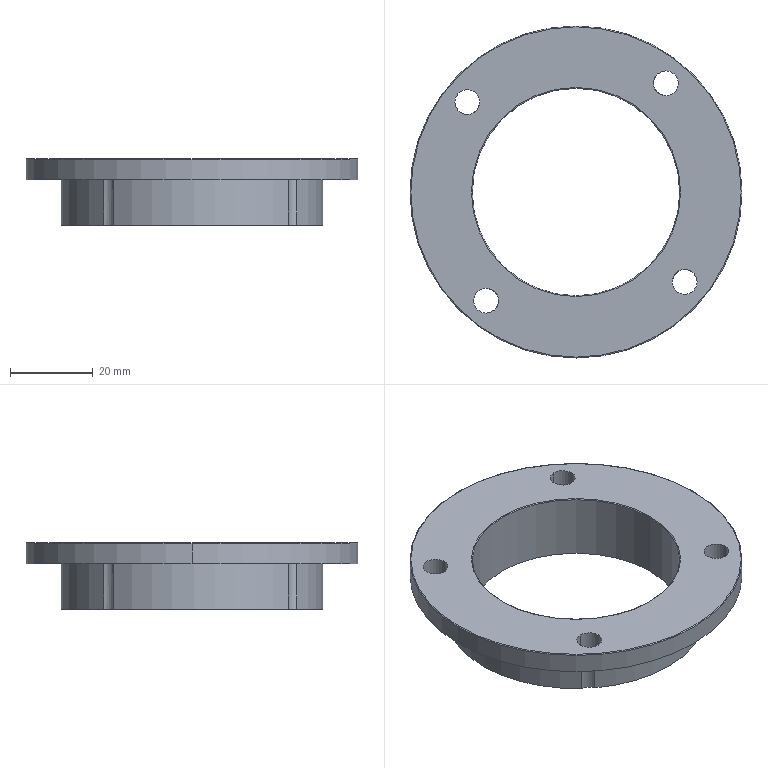Part | SolidWorks | 1 solid | 24 faces | box 80 x 80 x 16 mm | volume 27390 mm3 | cylinder 17 | torus 4 | plane 3 | commonest cylinder face diameters 6 x8 63 x5 50 x2 80 x2
STEP:
#1=CARTESIAN_POINT('',(325.,0.,69.8));
#2=VERTEX_POINT('',#1);
#3=CARTESIAN_POINT('',(275.,0.,69.8));
#4=VERTEX_POINT('',#3);
#5=CARTESIAN_POINT('',(300.,0.,69.8));
#6=DIRECTION('',(0.,0.,1.));
#7=DIRECTION('',(1.,0.009983,0.));
#8=AXIS2_PLACEMENT_3D('',#5,#6,#7);
#9=CIRCLE('',#8,25.);
#10=EDGE_CURVE('',#2,#4,#9,.T.);
#11=ORIENTED_EDGE('',*,*,#10,.F.);
#12=CARTESIAN_POINT('',(325.2,0.,70.));
#13=VERTEX_POINT('',#12);
#14=CARTESIAN_POINT('',(325.2,0.,69.8));
#15=DIRECTION('',(0.,1.,0.));
#16=DIRECTION('',(-1.,0.,0.));
#17=AXIS2_PLACEMENT_3D('',#14,#15,#16);
#18=CIRCLE('',#17,0.2);
#19=EDGE_CURVE('',#2,#13,#18,.T.);
#20=ORIENTED_EDGE('',*,*,#19,.T.);
#21=CARTESIAN_POINT('',(274.8,0.,70.));
#22=VERTEX_POINT('',#21);
#23=CARTESIAN_POINT('',(300.,0.,70.));
#24=DIRECTION('',(0.,0.,1.));
#25=DIRECTION('',(1.,0.,0.));
#26=AXIS2_PLACEMENT_3D('',#23,#24,#25);
#27=CIRCLE('',#26,25.2);
#28=EDGE_CURVE('',#13,#22,#27,.T.);
#29=ORIENTED_EDGE('',*,*,#28,.T.);
#30=CARTESIAN_POINT('',(274.8,0.,69.8));
#31=DIRECTION('',(0.,-1.,0.));
#32=DIRECTION('',(1.,0.,0.));
#33=AXIS2_PLACEMENT_3D('',#30,#31,#32);
#34=CIRCLE('',#33,0.2);
#35=EDGE_CURVE('',#4,#22,#34,.T.);
#36=ORIENTED_EDGE('',*,*,#35,.F.);
#37=EDGE_LOOP('',(#11,#20,#29,#36));
#38=FACE_OUTER_BOUND('',#37,.T.);
#39=CARTESIAN_POINT('',(300.,0.,69.8));
#40=DIRECTION('',(0.,0.,1.));
#41=DIRECTION('',(-1.,-0.009983,0.));
#42=AXIS2_PLACEMENT_3D('',#39,#40,#41);
#43=TOROIDAL_SURFACE('',#42,25.2,0.2);
#44=ADVANCED_FACE('',(#38),#43,.T.);
#45=CARTESIAN_POINT('',(300.,0.,69.8));
#46=DIRECTION('',(0.,0.,1.));
#47=DIRECTION('',(-1.,-0.009983,0.));
#48=AXIS2_PLACEMENT_3D('',#45,#46,#47);
#49=CIRCLE('',#48,25.);
#50=EDGE_CURVE('',#4,#2,#49,.T.);
#51=ORIENTED_EDGE('',*,*,#50,.F.);
#52=ORIENTED_EDGE('',*,*,#35,.T.);
#53=CARTESIAN_POINT('',(300.,0.,70.));
#54=DIRECTION('',(0.,0.,1.));
#55=DIRECTION('',(-1.,0.,0.));
#56=AXIS2_PLACEMENT_3D('',#53,#54,#55);
#57=CIRCLE('',#56,25.2);
#58=EDGE_CURVE('',#22,#13,#57,.T.);
#59=ORIENTED_EDGE('',*,*,#58,.T.);
#60=ORIENTED_EDGE('',*,*,#19,.F.);
#61=EDGE_LOOP('',(#51,#52,#59,#60));
#62=FACE_OUTER_BOUND('',#61,.T.);
#63=CARTESIAN_POINT('',(300.,0.,69.8));
#64=DIRECTION('',(0.,0.,1.));
#65=DIRECTION('',(1.,0.009983,0.));
#66=AXIS2_PLACEMENT_3D('',#63,#64,#65);
#67=TOROIDAL_SURFACE('',#66,25.2,0.2);
#68=ADVANCED_FACE('',(#62),#67,.T.);
#69=CARTESIAN_POINT('',(325.,0.,54.));
#70=VERTEX_POINT('',#69);
#71=CARTESIAN_POINT('',(275.,0.,54.));
#72=VERTEX_POINT('',#71);
#73=CARTESIAN_POINT('',(300.,0.,54.));
#74=DIRECTION('',(0.,0.,-1.));
#75=DIRECTION('',(1.,0.,0.));
#76=AXIS2_PLACEMENT_3D('',#73,#74,#75);
#77=CIRCLE('',#76,25.);
#78=EDGE_CURVE('',#70,#72,#77,.T.);
#79=ORIENTED_EDGE('',*,*,#78,.T.);
#80=CARTESIAN_POINT('',(275.,0.,54.));
#81=DIRECTION('',(0.,0.,1.));
#82=VECTOR('',#81,1000.);
#83=LINE('',#80,#82);
#84=EDGE_CURVE('',#72,#4,#83,.T.);
#85=ORIENTED_EDGE('',*,*,#84,.T.);
#86=ORIENTED_EDGE('',*,*,#50,.T.);
#87=CARTESIAN_POINT('',(325.,0.,54.));
#88=DIRECTION('',(0.,0.,1.));
#89=VECTOR('',#88,1000.);
#90=LINE('',#87,#89);
#91=EDGE_CURVE('',#70,#2,#90,.T.);
#92=ORIENTED_EDGE('',*,*,#91,.F.);
#93=EDGE_LOOP('',(#79,#85,#86,#92));
#94=FACE_OUTER_BOUND('',#93,.T.);
#95=CARTESIAN_POINT('',(300.,0.,70.));
#96=DIRECTION('',(0.,0.,1.));
#97=DIRECTION('',(1.,0.,0.));
#98=AXIS2_PLACEMENT_3D('',#95,#96,#97);
#99=CYLINDRICAL_SURFACE('',#98,25.);
#100=ADVANCED_FACE('',(#94),#99,.F.);
#101=CARTESIAN_POINT('',(300.,0.,54.));
#102=DIRECTION('',(0.,0.,-1.));
#103=DIRECTION('',(-1.,0.,0.));
#104=AXIS2_PLACEMENT_3D('',#101,#102,#103);
#105=CIRCLE('',#104,25.);
#106=EDGE_CURVE('',#72,#70,#105,.T.);
#107=ORIENTED_EDGE('',*,*,#106,.T.);
#108=ORIENTED_EDGE('',*,*,#91,.T.);
#109=ORIENTED_EDGE('',*,*,#10,.T.);
#110=ORIENTED_EDGE('',*,*,#84,.F.);
#111=EDGE_LOOP('',(#107,#108,#109,#110));
#112=FACE_OUTER_BOUND('',#111,.T.);
#113=CARTESIAN_POINT('',(300.,0.,70.));
#114=DIRECTION('',(0.,0.,1.));
#115=DIRECTION('',(1.,0.,0.));
#116=AXIS2_PLACEMENT_3D('',#113,#114,#115);
#117=CYLINDRICAL_SURFACE('',#116,25.);
#118=ADVANCED_FACE('',(#112),#117,.F.);
#119=CARTESIAN_POINT('',(331.5,0.,54.));
#120=VERTEX_POINT('',#119);
#121=CARTESIAN_POINT('',(321.283,23.223,54.));
#122=VERTEX_POINT('',#121);
#123=CARTESIAN_POINT('',(300.,0.,54.));
#124=DIRECTION('',(0.,0.,1.));
#125=DIRECTION('',(1.,0.,0.));
#126=AXIS2_PLACEMENT_3D('',#123,#124,#125);
#127=CIRCLE('',#126,31.5);
#128=EDGE_CURVE('',#120,#122,#127,.T.);
#129=ORIENTED_EDGE('',*,*,#128,.T.);
#130=CARTESIAN_POINT('',(321.283,23.223,65.));
#131=VERTEX_POINT('',#130);
#132=CARTESIAN_POINT('',(321.283,23.223,54.));
#133=DIRECTION('',(0.,0.,1.));
#134=VECTOR('',#133,1000.);
#135=LINE('',#132,#134);
#136=EDGE_CURVE('',#122,#131,#135,.T.);
#137=ORIENTED_EDGE('',*,*,#136,.T.);
#138=CARTESIAN_POINT('',(331.5,0.,65.));
#139=VERTEX_POINT('',#138);
#140=CARTESIAN_POINT('',(300.,0.,65.));
#141=DIRECTION('',(0.,0.,-1.));
#142=DIRECTION('',(0.6756,0.7372,0.));
#143=AXIS2_PLACEMENT_3D('',#140,#141,#142);
#144=CIRCLE('',#143,31.5);
#145=EDGE_CURVE('',#131,#139,#144,.T.);
#146=ORIENTED_EDGE('',*,*,#145,.T.);
#147=CARTESIAN_POINT('',(331.5,0.,65.));
#148=DIRECTION('',(0.,0.,-1.));
#149=VECTOR('',#148,1000.);
#150=LINE('',#147,#149);
#151=EDGE_CURVE('',#139,#120,#150,.T.);
#152=ORIENTED_EDGE('',*,*,#151,.T.);
#153=EDGE_LOOP('',(#129,#137,#146,#152));
#154=FACE_OUTER_BOUND('',#153,.T.);
#155=CARTESIAN_POINT('',(300.,0.,70.));
#156=DIRECTION('',(0.,0.,1.));
#157=DIRECTION('',(1.,0.,0.));
#158=AXIS2_PLACEMENT_3D('',#155,#156,#157);
#159=CYLINDRICAL_SURFACE('',#158,31.5);
#160=ADVANCED_FACE('',(#154),#159,.T.);
#161=ORIENTED_EDGE('',*,*,#151,.F.);
#162=CARTESIAN_POINT('',(325.257,-18.824,65.));
#163=VERTEX_POINT('',#162);
#164=CARTESIAN_POINT('',(300.,0.,65.));
#165=DIRECTION('',(0.,0.,-1.));
#166=DIRECTION('',(1.,0.,0.));
#167=AXIS2_PLACEMENT_3D('',#164,#165,#166);
#168=CIRCLE('',#167,31.5);
#169=EDGE_CURVE('',#139,#163,#168,.T.);
#170=ORIENTED_EDGE('',*,*,#169,.T.);
#171=CARTESIAN_POINT('',(325.257,-18.824,54.));
#172=VERTEX_POINT('',#171);
#173=CARTESIAN_POINT('',(325.257,-18.824,65.));
#174=DIRECTION('',(0.,0.,-1.));
#175=VECTOR('',#174,1000.);
#176=LINE('',#173,#175);
#177=EDGE_CURVE('',#163,#172,#176,.T.);
#178=ORIENTED_EDGE('',*,*,#177,.T.);
#179=CARTESIAN_POINT('',(300.,0.,54.));
#180=DIRECTION('',(0.,0.,1.));
#181=DIRECTION('',(0.8018,-0.5976,0.));
#182=AXIS2_PLACEMENT_3D('',#179,#180,#181);
#183=CIRCLE('',#182,31.5);
#184=EDGE_CURVE('',#172,#120,#183,.T.);
#185=ORIENTED_EDGE('',*,*,#184,.T.);
#186=EDGE_LOOP('',(#161,#170,#178,#185));
#187=FACE_OUTER_BOUND('',#186,.T.);
#188=CARTESIAN_POINT('',(300.,0.,70.));
#189=DIRECTION('',(0.,0.,1.));
#190=DIRECTION('',(1.,0.,0.));
#191=AXIS2_PLACEMENT_3D('',#188,#189,#190);
#192=CYLINDRICAL_SURFACE('',#191,31.5);
#193=ADVANCED_FACE('',(#187),#192,.T.);
#194=CARTESIAN_POINT('',(323.197,-21.672,70.));
#195=VERTEX_POINT('',#194);
#196=CARTESIAN_POINT('',(329.197,-21.672,70.));
#197=VERTEX_POINT('',#196);
#198=CARTESIAN_POINT('',(326.197,-21.672,70.));
#199=DIRECTION('',(0.,0.,1.));
#200=DIRECTION('',(-1.,0.,0.));
#201=AXIS2_PLACEMENT_3D('',#198,#199,#200);
#202=CIRCLE('',#201,3.);
#203=EDGE_CURVE('',#195,#197,#202,.T.);
#204=ORIENTED_EDGE('',*,*,#203,.T.);
#205=CARTESIAN_POINT('',(329.197,-21.672,65.));
#206=VERTEX_POINT('',#205);
#207=CARTESIAN_POINT('',(329.197,-21.672,65.));
#208=DIRECTION('',(0.,0.,1.));
#209=VECTOR('',#208,1000.);
#210=LINE('',#207,#209);
#211=EDGE_CURVE('',#206,#197,#210,.T.);
#212=ORIENTED_EDGE('',*,*,#211,.F.);
#213=CARTESIAN_POINT('',(323.197,-21.672,65.));
#214=VERTEX_POINT('',#213);
#215=CARTESIAN_POINT('',(326.197,-21.672,65.));
#216=DIRECTION('',(0.,0.,-1.));
#217=DIRECTION('',(1.,0.,0.));
#218=AXIS2_PLACEMENT_3D('',#215,#216,#217);
#219=CIRCLE('',#218,3.);
#220=EDGE_CURVE('',#206,#214,#219,.T.);
#221=ORIENTED_EDGE('',*,*,#220,.T.);
#222=CARTESIAN_POINT('',(323.197,-21.672,65.));
#223=DIRECTION('',(0.,0.,1.));
#224=VECTOR('',#223,1000.);
#225=LINE('',#222,#224);
#226=EDGE_CURVE('',#214,#195,#225,.T.);
#227=ORIENTED_EDGE('',*,*,#226,.T.);
#228=EDGE_LOOP('',(#204,#212,#221,#227));
#229=FACE_OUTER_BOUND('',#228,.T.);
#230=CARTESIAN_POINT('',(326.197,-21.672,70.));
#231=DIRECTION('',(0.,0.,1.));
#232=DIRECTION('',(-1.,0.,0.));
#233=AXIS2_PLACEMENT_3D('',#230,#231,#232);
#234=CYLINDRICAL_SURFACE('',#233,3.);
#235=ADVANCED_FACE('',(#229),#234,.F.);
#236=CARTESIAN_POINT('',(326.197,-21.672,70.));
#237=DIRECTION('',(0.,0.,1.));
#238=DIRECTION('',(1.,0.,0.));
#239=AXIS2_PLACEMENT_3D('',#236,#237,#238);
#240=CIRCLE('',#239,3.);
#241=EDGE_CURVE('',#197,#195,#240,.T.);
#242=ORIENTED_EDGE('',*,*,#241,.T.);
#243=ORIENTED_EDGE('',*,*,#226,.F.);
#244=CARTESIAN_POINT('',(323.223,-21.283,65.));
#245=VERTEX_POINT('',#244);
#246=CARTESIAN_POINT('',(326.197,-21.672,65.));
#247=DIRECTION('',(0.,0.,-1.));
#248=DIRECTION('',(-1.,0.,0.));
#249=AXIS2_PLACEMENT_3D('',#246,#247,#248);
#250=CIRCLE('',#249,3.);
#251=EDGE_CURVE('',#214,#245,#250,.T.);
#252=ORIENTED_EDGE('',*,*,#251,.T.);
#253=CARTESIAN_POINT('',(323.223,-21.283,54.));
#254=VERTEX_POINT('',#253);
#255=CARTESIAN_POINT('',(323.223,-21.283,54.));
#256=DIRECTION('',(0.,0.,1.));
#257=VECTOR('',#256,1000.);
#258=LINE('',#255,#257);
#259=EDGE_CURVE('',#254,#245,#258,.T.);
#260=ORIENTED_EDGE('',*,*,#259,.F.);
#261=CARTESIAN_POINT('',(326.197,-21.672,54.));
#262=DIRECTION('',(0.,0.,-1.));
#263=DIRECTION('',(-0.9915,0.13,0.));
#264=AXIS2_PLACEMENT_3D('',#261,#262,#263);
#265=CIRCLE('',#264,3.);
#266=EDGE_CURVE('',#254,#172,#265,.T.);
#267=ORIENTED_EDGE('',*,*,#266,.T.);
#268=ORIENTED_EDGE('',*,*,#177,.F.);
#269=CARTESIAN_POINT('',(326.197,-21.672,65.));
#270=DIRECTION('',(0.,0.,-1.));
#271=DIRECTION('',(-0.3134,0.9496,0.));
#272=AXIS2_PLACEMENT_3D('',#269,#270,#271);
#273=CIRCLE('',#272,3.);
#274=EDGE_CURVE('',#163,#206,#273,.T.);
#275=ORIENTED_EDGE('',*,*,#274,.T.);
#276=ORIENTED_EDGE('',*,*,#211,.T.);
#277=EDGE_LOOP('',(#242,#243,#252,#260,#267,#268,#275,#276));
#278=FACE_OUTER_BOUND('',#277,.T.);
#279=CARTESIAN_POINT('',(326.197,-21.672,70.));
#280=DIRECTION('',(0.,0.,1.));
#281=DIRECTION('',(-1.,0.,0.));
#282=AXIS2_PLACEMENT_3D('',#279,#280,#281);
#283=CYLINDRICAL_SURFACE('',#282,3.);
#284=ADVANCED_FACE('',(#278),#283,.F.);
#285=ORIENTED_EDGE('',*,*,#78,.F.);
#286=ORIENTED_EDGE('',*,*,#106,.F.);
#287=EDGE_LOOP('',(#285,#286));
#288=FACE_BOUND('',#287,.T.);
#289=CARTESIAN_POINT('',(274.743,18.824,54.));
#290=VERTEX_POINT('',#289);
#291=CARTESIAN_POINT('',(278.717,-23.223,54.));
#292=VERTEX_POINT('',#291);
#293=CARTESIAN_POINT('',(300.,0.,54.));
#294=DIRECTION('',(0.,0.,1.));
#295=DIRECTION('',(-1.,0.,0.));
#296=AXIS2_PLACEMENT_3D('',#293,#294,#295);
#297=CIRCLE('',#296,31.5);
#298=EDGE_CURVE('',#290,#292,#297,.T.);
#299=ORIENTED_EDGE('',*,*,#298,.F.);
#300=CARTESIAN_POINT('',(276.777,21.283,54.));
#301=VERTEX_POINT('',#300);
#302=CARTESIAN_POINT('',(273.803,21.672,54.));
#303=DIRECTION('',(0.,0.,-1.));
#304=DIRECTION('',(0.9915,-0.13,0.));
#305=AXIS2_PLACEMENT_3D('',#302,#303,#304);
#306=CIRCLE('',#305,3.);
#307=EDGE_CURVE('',#301,#290,#306,.T.);
#308=ORIENTED_EDGE('',*,*,#307,.F.);
#309=CARTESIAN_POINT('',(318.824,25.257,54.));
#310=VERTEX_POINT('',#309);
#311=CARTESIAN_POINT('',(300.,0.,54.));
#312=DIRECTION('',(0.,0.,1.));
#313=DIRECTION('',(0.5976,0.8018,0.));
#314=AXIS2_PLACEMENT_3D('',#311,#312,#313);
#315=CIRCLE('',#314,31.5);
#316=EDGE_CURVE('',#310,#301,#315,.T.);
#317=ORIENTED_EDGE('',*,*,#316,.F.);
#318=CARTESIAN_POINT('',(321.672,26.197,54.));
#319=DIRECTION('',(0.,0.,-1.));
#320=DIRECTION('',(-0.13,-0.9915,0.));
#321=AXIS2_PLACEMENT_3D('',#318,#319,#320);
#322=CIRCLE('',#321,3.);
#323=EDGE_CURVE('',#122,#310,#322,.T.);
#324=ORIENTED_EDGE('',*,*,#323,.F.);
#325=ORIENTED_EDGE('',*,*,#128,.F.);
#326=ORIENTED_EDGE('',*,*,#184,.F.);
#327=ORIENTED_EDGE('',*,*,#266,.F.);
#328=CARTESIAN_POINT('',(281.176,-25.257,54.));
#329=VERTEX_POINT('',#328);
#330=CARTESIAN_POINT('',(300.,0.,54.));
#331=DIRECTION('',(0.,0.,1.));
#332=DIRECTION('',(-0.5976,-0.8018,0.));
#333=AXIS2_PLACEMENT_3D('',#330,#331,#332);
#334=CIRCLE('',#333,31.5);
#335=EDGE_CURVE('',#329,#254,#334,.T.);
#336=ORIENTED_EDGE('',*,*,#335,.F.);
#337=CARTESIAN_POINT('',(278.328,-26.197,54.));
#338=DIRECTION('',(0.,0.,-1.));
#339=DIRECTION('',(0.13,0.9915,0.));
#340=AXIS2_PLACEMENT_3D('',#337,#338,#339);
#341=CIRCLE('',#340,3.);
#342=EDGE_CURVE('',#292,#329,#341,.T.);
#343=ORIENTED_EDGE('',*,*,#342,.F.);
#344=EDGE_LOOP('',(#299,#308,#317,#324,#325,#326,#327,#336,#343));
#345=FACE_OUTER_BOUND('',#344,.T.);
#346=CARTESIAN_POINT('',(300.497,29.496,54.));
#347=DIRECTION('',(0.,0.,1.));
#348=DIRECTION('',(1.,0.,0.));
#349=AXIS2_PLACEMENT_3D('',#346,#347,#348);
#350=PLANE('',#349);
#351=ADVANCED_FACE('',(#288,#345),#350,.F.);
#352=CARTESIAN_POINT('',(278.717,-23.223,65.));
#353=VERTEX_POINT('',#352);
#354=CARTESIAN_POINT('',(274.743,18.824,65.));
#355=VERTEX_POINT('',#354);
#356=CARTESIAN_POINT('',(300.,0.,65.));
#357=DIRECTION('',(0.,0.,-1.));
#358=DIRECTION('',(-0.6756,-0.7372,0.));
#359=AXIS2_PLACEMENT_3D('',#356,#357,#358);
#360=CIRCLE('',#359,31.5);
#361=EDGE_CURVE('',#353,#355,#360,.T.);
#362=ORIENTED_EDGE('',*,*,#361,.T.);
#363=CARTESIAN_POINT('',(274.743,18.824,65.));
#364=DIRECTION('',(0.,0.,-1.));
#365=VECTOR('',#364,1000.);
#366=LINE('',#363,#365);
#367=EDGE_CURVE('',#355,#290,#366,.T.);
#368=ORIENTED_EDGE('',*,*,#367,.T.);
#369=ORIENTED_EDGE('',*,*,#298,.T.);
#370=CARTESIAN_POINT('',(278.717,-23.223,54.));
#371=DIRECTION('',(0.,0.,1.));
#372=VECTOR('',#371,1000.);
#373=LINE('',#370,#372);
#374=EDGE_CURVE('',#292,#353,#373,.T.);
#375=ORIENTED_EDGE('',*,*,#374,.T.);
#376=EDGE_LOOP('',(#362,#368,#369,#375));
#377=FACE_OUTER_BOUND('',#376,.T.);
#378=CARTESIAN_POINT('',(300.,0.,70.));
#379=DIRECTION('',(0.,0.,1.));
#380=DIRECTION('',(1.,0.,0.));
#381=AXIS2_PLACEMENT_3D('',#378,#379,#380);
#382=CYLINDRICAL_SURFACE('',#381,31.5);
#383=ADVANCED_FACE('',(#377),#382,.T.);
#384=CARTESIAN_POINT('',(276.803,21.672,70.));
#385=VERTEX_POINT('',#384);
#386=CARTESIAN_POINT('',(270.803,21.672,70.));
#387=VERTEX_POINT('',#386);
#388=CARTESIAN_POINT('',(273.803,21.672,70.));
#389=DIRECTION('',(0.,0.,1.));
#390=DIRECTION('',(1.,0.,0.));
#391=AXIS2_PLACEMENT_3D('',#388,#389,#390);
#392=CIRCLE('',#391,3.);
#393=EDGE_CURVE('',#385,#387,#392,.T.);
#394=ORIENTED_EDGE('',*,*,#393,.T.);
#395=CARTESIAN_POINT('',(270.803,21.672,65.));
#396=VERTEX_POINT('',#395);
#397=CARTESIAN_POINT('',(270.803,21.672,65.));
#398=DIRECTION('',(0.,0.,1.));
#399=VECTOR('',#398,1000.);
#400=LINE('',#397,#399);
#401=EDGE_CURVE('',#396,#387,#400,.T.);
#402=ORIENTED_EDGE('',*,*,#401,.F.);
#403=CARTESIAN_POINT('',(276.803,21.672,65.));
#404=VERTEX_POINT('',#403);
#405=CARTESIAN_POINT('',(273.803,21.672,65.));
#406=DIRECTION('',(0.,0.,-1.));
#407=DIRECTION('',(-1.,0.,0.));
#408=AXIS2_PLACEMENT_3D('',#405,#406,#407);
#409=CIRCLE('',#408,3.);
#410=EDGE_CURVE('',#396,#404,#409,.T.);
#411=ORIENTED_EDGE('',*,*,#410,.T.);
#412=CARTESIAN_POINT('',(276.803,21.672,65.));
#413=DIRECTION('',(0.,0.,1.));
#414=VECTOR('',#413,1000.);
#415=LINE('',#412,#414);
#416=EDGE_CURVE('',#404,#385,#415,.T.);
#417=ORIENTED_EDGE('',*,*,#416,.T.);
#418=EDGE_LOOP('',(#394,#402,#411,#417));
#419=FACE_OUTER_BOUND('',#418,.T.);
#420=CARTESIAN_POINT('',(273.803,21.672,70.));
#421=DIRECTION('',(0.,0.,1.));
#422=DIRECTION('',(1.,0.,0.));
#423=AXIS2_PLACEMENT_3D('',#420,#421,#422);
#424=CYLINDRICAL_SURFACE('',#423,3.);
#425=ADVANCED_FACE('',(#419),#424,.F.);
#426=CARTESIAN_POINT('',(273.803,21.672,70.));
#427=DIRECTION('',(0.,0.,1.));
#428=DIRECTION('',(-1.,0.,0.));
#429=AXIS2_PLACEMENT_3D('',#426,#427,#428);
#430=CIRCLE('',#429,3.);
#431=EDGE_CURVE('',#387,#385,#430,.T.);
#432=ORIENTED_EDGE('',*,*,#431,.T.);
#433=ORIENTED_EDGE('',*,*,#416,.F.);
#434=CARTESIAN_POINT('',(276.777,21.283,65.));
#435=VERTEX_POINT('',#434);
#436=CARTESIAN_POINT('',(273.803,21.672,65.));
#437=DIRECTION('',(0.,0.,-1.));
#438=DIRECTION('',(1.,0.,0.));
#439=AXIS2_PLACEMENT_3D('',#436,#437,#438);
#440=CIRCLE('',#439,3.);
#441=EDGE_CURVE('',#404,#435,#440,.T.);
#442=ORIENTED_EDGE('',*,*,#441,.T.);
#443=CARTESIAN_POINT('',(276.777,21.283,54.));
#444=DIRECTION('',(0.,0.,1.));
#445=VECTOR('',#444,1000.);
#446=LINE('',#443,#445);
#447=EDGE_CURVE('',#301,#435,#446,.T.);
#448=ORIENTED_EDGE('',*,*,#447,.F.);
#449=ORIENTED_EDGE('',*,*,#307,.T.);
#450=ORIENTED_EDGE('',*,*,#367,.F.);
#451=CARTESIAN_POINT('',(273.803,21.672,65.));
#452=DIRECTION('',(0.,0.,-1.));
#453=DIRECTION('',(0.3134,-0.9496,0.));
#454=AXIS2_PLACEMENT_3D('',#451,#452,#453);
#455=CIRCLE('',#454,3.);
#456=EDGE_CURVE('',#355,#396,#455,.T.);
#457=ORIENTED_EDGE('',*,*,#456,.T.);
#458=ORIENTED_EDGE('',*,*,#401,.T.);
#459=EDGE_LOOP('',(#432,#433,#442,#448,#449,#450,#457,#458));
#460=FACE_OUTER_BOUND('',#459,.T.);
#461=CARTESIAN_POINT('',(273.803,21.672,70.));
#462=DIRECTION('',(0.,0.,1.));
#463=DIRECTION('',(1.,0.,0.));
#464=AXIS2_PLACEMENT_3D('',#461,#462,#463);
#465=CYLINDRICAL_SURFACE('',#464,3.);
#466=ADVANCED_FACE('',(#460),#465,.F.);
#467=ORIENTED_EDGE('',*,*,#316,.T.);
#468=ORIENTED_EDGE('',*,*,#447,.T.);
#469=CARTESIAN_POINT('',(318.824,25.257,65.));
#470=VERTEX_POINT('',#469);
#471=CARTESIAN_POINT('',(300.,0.,65.));
#472=DIRECTION('',(0.,0.,-1.));
#473=DIRECTION('',(-0.7372,0.6756,0.));
#474=AXIS2_PLACEMENT_3D('',#471,#472,#473);
#475=CIRCLE('',#474,31.5);
#476=EDGE_CURVE('',#435,#470,#475,.T.);
#477=ORIENTED_EDGE('',*,*,#476,.T.);
#478=CARTESIAN_POINT('',(318.824,25.257,65.));
#479=DIRECTION('',(0.,0.,-1.));
#480=VECTOR('',#479,1000.);
#481=LINE('',#478,#480);
#482=EDGE_CURVE('',#470,#310,#481,.T.);
#483=ORIENTED_EDGE('',*,*,#482,.T.);
#484=EDGE_LOOP('',(#467,#468,#477,#483));
#485=FACE_OUTER_BOUND('',#484,.T.);
#486=CARTESIAN_POINT('',(300.,0.,70.));
#487=DIRECTION('',(0.,0.,1.));
#488=DIRECTION('',(1.,0.,0.));
#489=AXIS2_PLACEMENT_3D('',#486,#487,#488);
#490=CYLINDRICAL_SURFACE('',#489,31.5);
#491=ADVANCED_FACE('',(#485),#490,.T.);
#492=CARTESIAN_POINT('',(321.672,23.197,70.));
#493=VERTEX_POINT('',#492);
#494=CARTESIAN_POINT('',(321.672,29.197,70.));
#495=VERTEX_POINT('',#494);
#496=CARTESIAN_POINT('',(321.672,26.197,70.));
#497=DIRECTION('',(0.,0.,1.));
#498=DIRECTION('',(0.,-1.,0.));
#499=AXIS2_PLACEMENT_3D('',#496,#497,#498);
#500=CIRCLE('',#499,3.);
#501=EDGE_CURVE('',#493,#495,#500,.T.);
#502=ORIENTED_EDGE('',*,*,#501,.T.);
#503=CARTESIAN_POINT('',(321.672,29.197,65.));
#504=VERTEX_POINT('',#503);
#505=CARTESIAN_POINT('',(321.672,29.197,65.));
#506=DIRECTION('',(0.,0.,1.));
#507=VECTOR('',#506,1000.);
#508=LINE('',#505,#507);
#509=EDGE_CURVE('',#504,#495,#508,.T.);
#510=ORIENTED_EDGE('',*,*,#509,.F.);
#511=CARTESIAN_POINT('',(321.672,23.197,65.));
#512=VERTEX_POINT('',#511);
#513=CARTESIAN_POINT('',(321.672,26.197,65.));
#514=DIRECTION('',(0.,0.,-1.));
#515=DIRECTION('',(0.,1.,0.));
#516=AXIS2_PLACEMENT_3D('',#513,#514,#515);
#517=CIRCLE('',#516,3.);
#518=EDGE_CURVE('',#504,#512,#517,.T.);
#519=ORIENTED_EDGE('',*,*,#518,.T.);
#520=CARTESIAN_POINT('',(321.672,23.197,65.));
#521=DIRECTION('',(0.,0.,1.));
#522=VECTOR('',#521,1000.);
#523=LINE('',#520,#522);
#524=EDGE_CURVE('',#512,#493,#523,.T.);
#525=ORIENTED_EDGE('',*,*,#524,.T.);
#526=EDGE_LOOP('',(#502,#510,#519,#525));
#527=FACE_OUTER_BOUND('',#526,.T.);
#528=CARTESIAN_POINT('',(321.672,26.197,70.));
#529=DIRECTION('',(0.,0.,1.));
#530=DIRECTION('',(0.,-1.,0.));
#531=AXIS2_PLACEMENT_3D('',#528,#529,#530);
#532=CYLINDRICAL_SURFACE('',#531,3.);
#533=ADVANCED_FACE('',(#527),#532,.F.);
#534=CARTESIAN_POINT('',(321.672,26.197,70.));
#535=DIRECTION('',(0.,0.,1.));
#536=DIRECTION('',(0.,1.,0.));
#537=AXIS2_PLACEMENT_3D('',#534,#535,#536);
#538=CIRCLE('',#537,3.);
#539=EDGE_CURVE('',#495,#493,#538,.T.);
#540=ORIENTED_EDGE('',*,*,#539,.T.);
#541=ORIENTED_EDGE('',*,*,#524,.F.);
#542=CARTESIAN_POINT('',(321.672,26.197,65.));
#543=DIRECTION('',(0.,0.,-1.));
#544=DIRECTION('',(0.,-1.,0.));
#545=AXIS2_PLACEMENT_3D('',#542,#543,#544);
#546=CIRCLE('',#545,3.);
#547=EDGE_CURVE('',#512,#131,#546,.T.);
#548=ORIENTED_EDGE('',*,*,#547,.T.);
#549=ORIENTED_EDGE('',*,*,#136,.F.);
#550=ORIENTED_EDGE('',*,*,#323,.T.);
#551=ORIENTED_EDGE('',*,*,#482,.F.);
#552=CARTESIAN_POINT('',(321.672,26.197,65.));
#553=DIRECTION('',(0.,0.,-1.));
#554=DIRECTION('',(-0.9496,-0.3134,0.));
#555=AXIS2_PLACEMENT_3D('',#552,#553,#554);
#556=CIRCLE('',#555,3.);
#557=EDGE_CURVE('',#470,#504,#556,.T.);
#558=ORIENTED_EDGE('',*,*,#557,.T.);
#559=ORIENTED_EDGE('',*,*,#509,.T.);
#560=EDGE_LOOP('',(#540,#541,#548,#549,#550,#551,#558,#559));
#561=FACE_OUTER_BOUND('',#560,.T.);
#562=CARTESIAN_POINT('',(321.672,26.197,70.));
#563=DIRECTION('',(0.,0.,1.));
#564=DIRECTION('',(0.,-1.,0.));
#565=AXIS2_PLACEMENT_3D('',#562,#563,#564);
#566=CYLINDRICAL_SURFACE('',#565,3.);
#567=ADVANCED_FACE('',(#561),#566,.F.);
#568=ORIENTED_EDGE('',*,*,#58,.F.);
#569=ORIENTED_EDGE('',*,*,#28,.F.);
#570=EDGE_LOOP('',(#568,#569));
#571=FACE_BOUND('',#570,.T.);
#572=ORIENTED_EDGE('',*,*,#393,.F.);
#573=ORIENTED_EDGE('',*,*,#431,.F.);
#574=EDGE_LOOP('',(#572,#573));
#575=FACE_BOUND('',#574,.T.);
#576=CARTESIAN_POINT('',(278.328,-23.197,70.));
#577=VERTEX_POINT('',#576);
#578=CARTESIAN_POINT('',(278.328,-29.197,70.));
#579=VERTEX_POINT('',#578);
#580=CARTESIAN_POINT('',(278.328,-26.197,70.));
#581=DIRECTION('',(0.,0.,1.));
#582=DIRECTION('',(0.,1.,0.));
#583=AXIS2_PLACEMENT_3D('',#580,#581,#582);
#584=CIRCLE('',#583,3.);
#585=EDGE_CURVE('',#577,#579,#584,.T.);
#586=ORIENTED_EDGE('',*,*,#585,.F.);
#587=CARTESIAN_POINT('',(278.328,-26.197,70.));
#588=DIRECTION('',(0.,0.,1.));
#589=DIRECTION('',(0.,-1.,0.));
#590=AXIS2_PLACEMENT_3D('',#587,#588,#589);
#591=CIRCLE('',#590,3.);
#592=EDGE_CURVE('',#579,#577,#591,.T.);
#593=ORIENTED_EDGE('',*,*,#592,.F.);
#594=EDGE_LOOP('',(#586,#593));
#595=FACE_BOUND('',#594,.T.);
#596=ORIENTED_EDGE('',*,*,#203,.F.);
#597=ORIENTED_EDGE('',*,*,#241,.F.);
#598=EDGE_LOOP('',(#596,#597));
#599=FACE_BOUND('',#598,.T.);
#600=ORIENTED_EDGE('',*,*,#501,.F.);
#601=ORIENTED_EDGE('',*,*,#539,.F.);
#602=EDGE_LOOP('',(#600,#601));
#603=FACE_BOUND('',#602,.T.);
#604=CARTESIAN_POINT('',(339.8,0.,70.));
#605=VERTEX_POINT('',#604);
#606=CARTESIAN_POINT('',(260.2,0.,70.));
#607=VERTEX_POINT('',#606);
#608=CARTESIAN_POINT('',(300.,0.,70.));
#609=DIRECTION('',(0.,0.,-1.));
#610=DIRECTION('',(1.,0.,0.));
#611=AXIS2_PLACEMENT_3D('',#608,#609,#610);
#612=CIRCLE('',#611,39.8);
#613=EDGE_CURVE('',#605,#607,#612,.T.);
#614=ORIENTED_EDGE('',*,*,#613,.F.);
#615=CARTESIAN_POINT('',(300.,0.,70.));
#616=DIRECTION('',(0.,0.,-1.));
#617=DIRECTION('',(-1.,0.,0.));
#618=AXIS2_PLACEMENT_3D('',#615,#616,#617);
#619=CIRCLE('',#618,39.8);
#620=EDGE_CURVE('',#607,#605,#619,.T.);
#621=ORIENTED_EDGE('',*,*,#620,.F.);
#622=EDGE_LOOP('',(#614,#621));
#623=FACE_OUTER_BOUND('',#622,.T.);
#624=CARTESIAN_POINT('',(0.,0.,70.));
#625=DIRECTION('',(0.,0.,1.));
#626=DIRECTION('',(1.,0.,0.));
#627=AXIS2_PLACEMENT_3D('',#624,#625,#626);
#628=PLANE('',#627);
#629=ADVANCED_FACE('',(#571,#575,#595,#599,#603,#623),#628,.T.);
#630=CARTESIAN_POINT('',(340.,0.,69.8));
#631=VERTEX_POINT('',#630);
#632=CARTESIAN_POINT('',(260.,0.,69.8));
#633=VERTEX_POINT('',#632);
#634=CARTESIAN_POINT('',(300.,0.,69.8));
#635=DIRECTION('',(0.,0.,-1.));
#636=DIRECTION('',(1.,0.,0.));
#637=AXIS2_PLACEMENT_3D('',#634,#635,#636);
#638=CIRCLE('',#637,40.);
#639=EDGE_CURVE('',#631,#633,#638,.T.);
#640=ORIENTED_EDGE('',*,*,#639,.F.);
#641=CARTESIAN_POINT('',(339.8,0.,69.8));
#642=DIRECTION('',(0.,-1.,0.));
#643=DIRECTION('',(1.,0.,0.));
#644=AXIS2_PLACEMENT_3D('',#641,#642,#643);
#645=CIRCLE('',#644,0.2);
#646=EDGE_CURVE('',#631,#605,#645,.T.);
#647=ORIENTED_EDGE('',*,*,#646,.T.);
#648=ORIENTED_EDGE('',*,*,#613,.T.);
#649=CARTESIAN_POINT('',(260.2,0.,69.8));
#650=DIRECTION('',(0.,1.,0.));
#651=DIRECTION('',(-1.,0.,0.));
#652=AXIS2_PLACEMENT_3D('',#649,#650,#651);
#653=CIRCLE('',#652,0.2);
#654=EDGE_CURVE('',#633,#607,#653,.T.);
#655=ORIENTED_EDGE('',*,*,#654,.F.);
#656=EDGE_LOOP('',(#640,#647,#648,#655));
#657=FACE_OUTER_BOUND('',#656,.T.);
#658=CARTESIAN_POINT('',(300.,0.,69.8));
#659=DIRECTION('',(0.,0.,1.));
#660=DIRECTION('',(-1.,0.004392,0.));
#661=AXIS2_PLACEMENT_3D('',#658,#659,#660);
#662=TOROIDAL_SURFACE('',#661,39.8,0.2);
#663=ADVANCED_FACE('',(#657),#662,.T.);
#664=CARTESIAN_POINT('',(300.,0.,69.8));
#665=DIRECTION('',(0.,0.,-1.));
#666=DIRECTION('',(-1.,0.,0.));
#667=AXIS2_PLACEMENT_3D('',#664,#665,#666);
#668=CIRCLE('',#667,40.);
#669=EDGE_CURVE('',#633,#631,#668,.T.);
#670=ORIENTED_EDGE('',*,*,#669,.F.);
#671=ORIENTED_EDGE('',*,*,#654,.T.);
#672=ORIENTED_EDGE('',*,*,#620,.T.);
#673=ORIENTED_EDGE('',*,*,#646,.F.);
#674=EDGE_LOOP('',(#670,#671,#672,#673));
#675=FACE_OUTER_BOUND('',#674,.T.);
#676=CARTESIAN_POINT('',(300.,0.,69.8));
#677=DIRECTION('',(0.,0.,1.));
#678=DIRECTION('',(1.,-0.004392,0.));
#679=AXIS2_PLACEMENT_3D('',#676,#677,#678);
#680=TOROIDAL_SURFACE('',#679,39.8,0.2);
#681=ADVANCED_FACE('',(#675),#680,.T.);
#682=CARTESIAN_POINT('',(340.,0.,65.));
#683=VERTEX_POINT('',#682);
#684=CARTESIAN_POINT('',(260.,0.,65.));
#685=VERTEX_POINT('',#684);
#686=CARTESIAN_POINT('',(300.,0.,65.));
#687=DIRECTION('',(0.,0.,1.));
#688=DIRECTION('',(1.,0.,0.));
#689=AXIS2_PLACEMENT_3D('',#686,#687,#688);
#690=CIRCLE('',#689,40.);
#691=EDGE_CURVE('',#683,#685,#690,.T.);
#692=ORIENTED_EDGE('',*,*,#691,.T.);
#693=CARTESIAN_POINT('',(260.,0.,69.8));
#694=DIRECTION('',(0.,0.,-1.));
#695=VECTOR('',#694,1000.);
#696=LINE('',#693,#695);
#697=EDGE_CURVE('',#633,#685,#696,.T.);
#698=ORIENTED_EDGE('',*,*,#697,.F.);
#699=ORIENTED_EDGE('',*,*,#669,.T.);
#700=CARTESIAN_POINT('',(340.,0.,69.8));
#701=DIRECTION('',(0.,0.,-1.));
#702=VECTOR('',#701,1000.);
#703=LINE('',#700,#702);
#704=EDGE_CURVE('',#631,#683,#703,.T.);
#705=ORIENTED_EDGE('',*,*,#704,.T.);
#706=EDGE_LOOP('',(#692,#698,#699,#705));
#707=FACE_OUTER_BOUND('',#706,.T.);
#708=CARTESIAN_POINT('',(300.,0.,65.));
#709=DIRECTION('',(0.,0.,1.));
#710=DIRECTION('',(1.,0.,0.));
#711=AXIS2_PLACEMENT_3D('',#708,#709,#710);
#712=CYLINDRICAL_SURFACE('',#711,40.);
#713=ADVANCED_FACE('',(#707),#712,.T.);
#714=CARTESIAN_POINT('',(300.,0.,65.));
#715=DIRECTION('',(0.,0.,1.));
#716=DIRECTION('',(-1.,0.,0.));
#717=AXIS2_PLACEMENT_3D('',#714,#715,#716);
#718=CIRCLE('',#717,40.);
#719=EDGE_CURVE('',#685,#683,#718,.T.);
#720=ORIENTED_EDGE('',*,*,#719,.T.);
#721=ORIENTED_EDGE('',*,*,#704,.F.);
#722=ORIENTED_EDGE('',*,*,#639,.T.);
#723=ORIENTED_EDGE('',*,*,#697,.T.);
#724=EDGE_LOOP('',(#720,#721,#722,#723));
#725=FACE_OUTER_BOUND('',#724,.T.);
#726=CARTESIAN_POINT('',(300.,0.,65.));
#727=DIRECTION('',(0.,0.,1.));
#728=DIRECTION('',(1.,0.,0.));
#729=AXIS2_PLACEMENT_3D('',#726,#727,#728);
#730=CYLINDRICAL_SURFACE('',#729,40.);
#731=ADVANCED_FACE('',(#725),#730,.T.);
#732=CARTESIAN_POINT('',(281.176,-25.257,65.));
#733=VERTEX_POINT('',#732);
#734=CARTESIAN_POINT('',(300.,0.,65.));
#735=DIRECTION('',(0.,0.,-1.));
#736=DIRECTION('',(0.7372,-0.6756,0.));
#737=AXIS2_PLACEMENT_3D('',#734,#735,#736);
#738=CIRCLE('',#737,31.5);
#739=EDGE_CURVE('',#245,#733,#738,.T.);
#740=ORIENTED_EDGE('',*,*,#739,.F.);
#741=ORIENTED_EDGE('',*,*,#251,.F.);
#742=ORIENTED_EDGE('',*,*,#220,.F.);
#743=ORIENTED_EDGE('',*,*,#274,.F.);
#744=ORIENTED_EDGE('',*,*,#169,.F.);
#745=ORIENTED_EDGE('',*,*,#145,.F.);
#746=ORIENTED_EDGE('',*,*,#547,.F.);
#747=ORIENTED_EDGE('',*,*,#518,.F.);
#748=ORIENTED_EDGE('',*,*,#557,.F.);
#749=ORIENTED_EDGE('',*,*,#476,.F.);
#750=ORIENTED_EDGE('',*,*,#441,.F.);
#751=ORIENTED_EDGE('',*,*,#410,.F.);
#752=ORIENTED_EDGE('',*,*,#456,.F.);
#753=ORIENTED_EDGE('',*,*,#361,.F.);
#754=CARTESIAN_POINT('',(278.328,-23.197,65.));
#755=VERTEX_POINT('',#754);
#756=CARTESIAN_POINT('',(278.328,-26.197,65.));
#757=DIRECTION('',(0.,0.,-1.));
#758=DIRECTION('',(0.,1.,0.));
#759=AXIS2_PLACEMENT_3D('',#756,#757,#758);
#760=CIRCLE('',#759,3.);
#761=EDGE_CURVE('',#755,#353,#760,.T.);
#762=ORIENTED_EDGE('',*,*,#761,.F.);
#763=CARTESIAN_POINT('',(278.328,-29.197,65.));
#764=VERTEX_POINT('',#763);
#765=CARTESIAN_POINT('',(278.328,-26.197,65.));
#766=DIRECTION('',(0.,0.,-1.));
#767=DIRECTION('',(0.,-1.,0.));
#768=AXIS2_PLACEMENT_3D('',#765,#766,#767);
#769=CIRCLE('',#768,3.);
#770=EDGE_CURVE('',#764,#755,#769,.T.);
#771=ORIENTED_EDGE('',*,*,#770,.F.);
#772=CARTESIAN_POINT('',(278.328,-26.197,65.));
#773=DIRECTION('',(0.,0.,-1.));
#774=DIRECTION('',(0.9496,0.3134,0.));
#775=AXIS2_PLACEMENT_3D('',#772,#773,#774);
#776=CIRCLE('',#775,3.);
#777=EDGE_CURVE('',#733,#764,#776,.T.);
#778=ORIENTED_EDGE('',*,*,#777,.F.);
#779=EDGE_LOOP('',(#740,#741,#742,#743,#744,#745,#746,#747,#748,#749,#750,#751,#752,#753,#762,#771,#778));
#780=FACE_BOUND('',#779,.T.);
#781=ORIENTED_EDGE('',*,*,#691,.F.);
#782=ORIENTED_EDGE('',*,*,#719,.F.);
#783=EDGE_LOOP('',(#781,#782));
#784=FACE_OUTER_BOUND('',#783,.T.);
#785=CARTESIAN_POINT('',(0.,0.,65.));
#786=DIRECTION('',(0.,0.,1.));
#787=DIRECTION('',(1.,0.,0.));
#788=AXIS2_PLACEMENT_3D('',#785,#786,#787);
#789=PLANE('',#788);
#790=ADVANCED_FACE('',(#780,#784),#789,.F.);
#791=ORIENTED_EDGE('',*,*,#585,.T.);
#792=CARTESIAN_POINT('',(278.328,-29.197,65.));
#793=DIRECTION('',(0.,0.,1.));
#794=VECTOR('',#793,1000.);
#795=LINE('',#792,#794);
#796=EDGE_CURVE('',#764,#579,#795,.T.);
#797=ORIENTED_EDGE('',*,*,#796,.F.);
#798=ORIENTED_EDGE('',*,*,#770,.T.);
#799=CARTESIAN_POINT('',(278.328,-23.197,65.));
#800=DIRECTION('',(0.,0.,1.));
#801=VECTOR('',#800,1000.);
#802=LINE('',#799,#801);
#803=EDGE_CURVE('',#755,#577,#802,.T.);
#804=ORIENTED_EDGE('',*,*,#803,.T.);
#805=EDGE_LOOP('',(#791,#797,#798,#804));
#806=FACE_OUTER_BOUND('',#805,.T.);
#807=CARTESIAN_POINT('',(278.328,-26.197,70.));
#808=DIRECTION('',(0.,0.,1.));
#809=DIRECTION('',(0.,1.,0.));
#810=AXIS2_PLACEMENT_3D('',#807,#808,#809);
#811=CYLINDRICAL_SURFACE('',#810,3.);
#812=ADVANCED_FACE('',(#806),#811,.F.);
#813=ORIENTED_EDGE('',*,*,#592,.T.);
#814=ORIENTED_EDGE('',*,*,#803,.F.);
#815=ORIENTED_EDGE('',*,*,#761,.T.);
#816=ORIENTED_EDGE('',*,*,#374,.F.);
#817=ORIENTED_EDGE('',*,*,#342,.T.);
#818=CARTESIAN_POINT('',(281.176,-25.257,65.));
#819=DIRECTION('',(0.,0.,-1.));
#820=VECTOR('',#819,1000.);
#821=LINE('',#818,#820);
#822=EDGE_CURVE('',#733,#329,#821,.T.);
#823=ORIENTED_EDGE('',*,*,#822,.F.);
#824=ORIENTED_EDGE('',*,*,#777,.T.);
#825=ORIENTED_EDGE('',*,*,#796,.T.);
#826=EDGE_LOOP('',(#813,#814,#815,#816,#817,#823,#824,#825));
#827=FACE_OUTER_BOUND('',#826,.T.);
#828=CARTESIAN_POINT('',(278.328,-26.197,70.));
#829=DIRECTION('',(0.,0.,1.));
#830=DIRECTION('',(0.,1.,0.));
#831=AXIS2_PLACEMENT_3D('',#828,#829,#830);
#832=CYLINDRICAL_SURFACE('',#831,3.);
#833=ADVANCED_FACE('',(#827),#832,.F.);
#834=ORIENTED_EDGE('',*,*,#335,.T.);
#835=ORIENTED_EDGE('',*,*,#259,.T.);
#836=ORIENTED_EDGE('',*,*,#739,.T.);
#837=ORIENTED_EDGE('',*,*,#822,.T.);
#838=EDGE_LOOP('',(#834,#835,#836,#837));
#839=FACE_OUTER_BOUND('',#838,.T.);
#840=CARTESIAN_POINT('',(300.,0.,70.));
#841=DIRECTION('',(0.,0.,1.));
#842=DIRECTION('',(1.,0.,0.));
#843=AXIS2_PLACEMENT_3D('',#840,#841,#842);
#844=CYLINDRICAL_SURFACE('',#843,31.5);
#845=ADVANCED_FACE('',(#839),#844,.T.);
#846=CLOSED_SHELL('',(#44,#68,#100,#118,#160,#193,#235,#284,#351,#383,#425,#466,#491,#533,#567,#629,#663,#681,#713,#731,#790,#812,#833,#845));
#847=MANIFOLD_SOLID_BREP('',#846);
#848=CARTESIAN_POINT('',(0.,0.,0.));
#849=DIRECTION('',(0.,0.,1.));
#850=DIRECTION('',(1.,0.,0.));
#851=AXIS2_PLACEMENT_3D('',#848,#849,#850);
#852=(LENGTH_UNIT()NAMED_UNIT(*)SI_UNIT(.MILLI.,.METRE.));
#853=UNCERTAINTY_MEASURE_WITH_UNIT(LENGTH_MEASURE(0.00001),#852,'','');
#854=(NAMED_UNIT(*)PLANE_ANGLE_UNIT()SI_UNIT($,.RADIAN.));
#855=(NAMED_UNIT(*)SI_UNIT($,.STERADIAN.)SOLID_ANGLE_UNIT());
#856=(GEOMETRIC_REPRESENTATION_CONTEXT(3)GLOBAL_UNCERTAINTY_ASSIGNED_CONTEXT((#853))GLOBAL_UNIT_ASSIGNED_CONTEXT((#852,#854,#855))REPRESENTATION_CONTEXT('',''));
#857=ADVANCED_BREP_SHAPE_REPRESENTATION('',(#847,#851),#856);